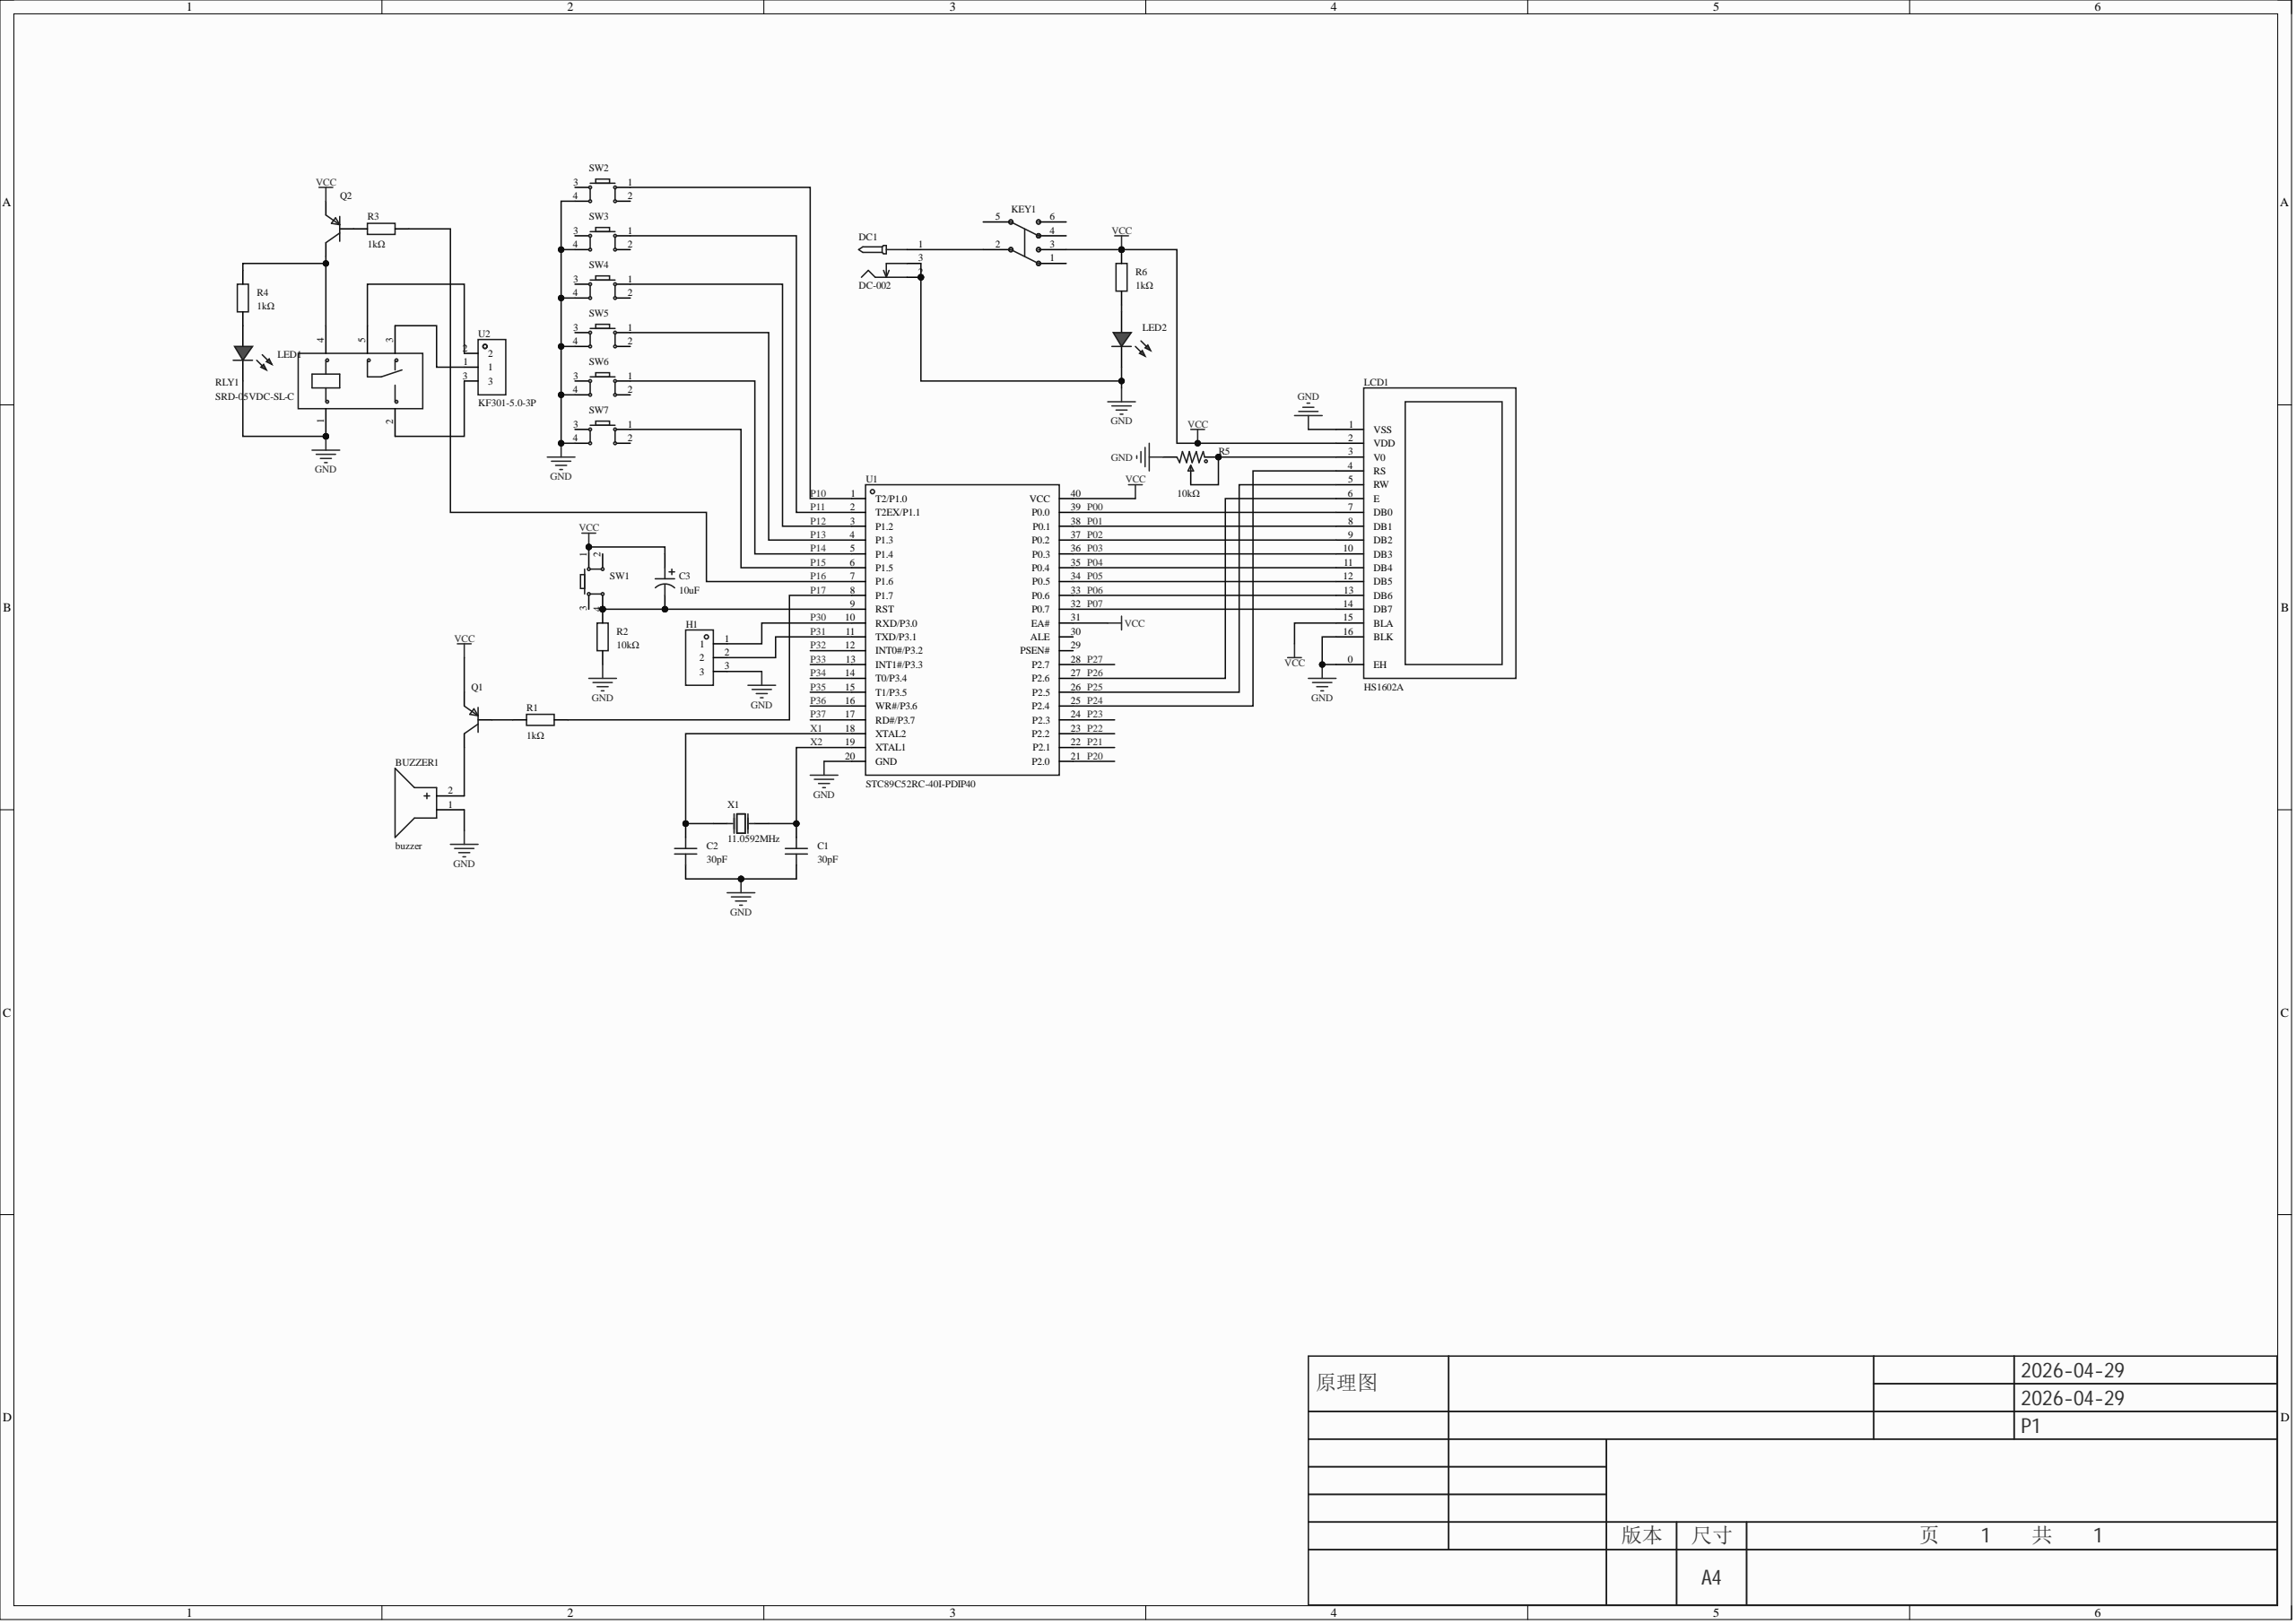Circuit board | Altium Designer | 29 parts | 37 nets
Bill of materials:
Comment,Description,Designator,Footprint,LibRef,Quantity
"buzzer","","BUZZER1","BUZ-TH_BD12.0-P6.00-D0.9-RD","buzzer","1"
"30pF","容值:30pF;精度:±10%;额定电压:25V;温度系数:C0G;","C1, C2","CAP-TH_L3.8-W2.5-P2.54-D0.50","C315C300K3G5TA7301","2"
"10uF","","C3","CAP-TH_BD5.0-P2.00-D0.8-FD-10UF50VC110GL","10UF50VC110GL","1"
"DC-002","","DC1","DC-IN-TH_DC-3510","DC-002","1"
"","","H1","HDR-TH_3P-P2.54-V-M","HDR-M_2.54_1x3P","1"
"无自锁开关 8.5×8.5 无声","6脚，8.5×8.5","KEY1","SW-TH_6P-L8.5-W8.5-P2.54","无自锁开关 8.5×8.5 无声","1"
"HS1602A","主控芯片:SPLC780;尺寸(inch):2;","LCD1","LCD1602","HS1602A","1"
"","","LED1, LED2","LED_TH-3mm","LED_TH-R_3mm","2"
"","","Q1, Q2","S8550P_TO-92","S8550_TO_PNP","2"
"1kΩ","","R1, R3, R4, R6","Res_1/8W","Res_AXIAL-1/8W","4"
"10kΩ","","R2","Res_1/8W","Res_AXIAL-1/8W","1"
"10kΩ","","R5","RES-ADJ-SMD_RM065-V1","RM065-103(10K)","1"
"SRD-05VDC-SL-C","线圈电压:5V;触点形式:一组转换:1C(单刀双掷-转换);触点容量(电阻负载):-;最大切换电压:250V@AC;最大切换电流:15A;","RLY1","RELAY-TH_SRD-XXVDC-XL-C","SRD-05VDC-SL-C","1"
"","","SW1, SW2, SW3, SW4, SW5, SW6, SW7","SW-TH_4P-L6.0-W6.0-P4.50-LS6.5","Key_TH_6x6x6","7"
"STC89C52RC-40I-PDIP40","CPU内核:51家族;CPU最大主频:-;","U1","DIP-40_L52.0-W13.7-P2.54-LS15.2-BL","STC89C52RC-40I-PDIP40","1"
"KF301-5.0-3P","结构:1x3P;间距:5mm;颜色:蓝色;安装方式:直插;排数:1;每排PIN数:3;额定电流:17A;额定电压:250V;线规 - AWG:14~22;线规 - 平方毫米:1.5;工作温度:-30℃~+120℃;","U2","CONN-TH_3P-P5.00_KF301-5.0-3P","KF301-5.0-3P","1"
"11.059MHz","晶振类型:直插晶振;频率:11.059MHz;常温频差:±20ppm;负载电容:30pF;","X1","OSC-TH_L11.1-W4.7-P4.88","9AC11059302060C3","1"
Netlist (Protel format):
[
BUZZER1
BUZ-TH_BD12.0-P6.00-D0.9-RD
buzzer



]
[
C1
CAP-TH_L3.8-W2.5-P2.54-D0.50
30pF



]
[
C2
CAP-TH_L3.8-W2.5-P2.54-D0.50
30pF



]
[
C3
CAP-TH_BD5.0-P2.00-D0.8-FD-10UF50VC110GL
10uF



]
[
DC1
DC-IN-TH_DC-3510
DC-002



]
[
H1
HDR-TH_3P-P2.54-V-M




]
[
KEY1
SW-TH_6P-L8.5-W8.5-P2.54
无自锁开关 8.5×8.5 无声



]
[
LCD1
LCD1602
HS1602A



]
[
LED1
LED_TH-3mm




]
[
LED2
LED_TH-3mm




]
[
Q1
S8550P_TO-92




]
[
Q2
S8550P_TO-92




]
[
R1
Res_1/8W
1kΩ



]
[
R2
Res_1/8W
10kΩ



]
[
R3
Res_1/8W
1kΩ



]
[
R4
Res_1/8W
1kΩ



]
[
R5
RES-ADJ-SMD_RM065-V1
10kΩ



]
[
R6
Res_1/8W
1kΩ



]
[
RLY1
RELAY-TH_SRD-XXVDC-XL-C
SRD-05VDC-SL-C



]
[
SW1
SW-TH_4P-L6.0-W6.0-P4.50-LS6.5




]
[
SW2
SW-TH_4P-L6.0-W6.0-P4.50-LS6.5




]
[
SW3
SW-TH_4P-L6.0-W6.0-P4.50-LS6.5




]
[
SW4
SW-TH_4P-L6.0-W6.0-P4.50-LS6.5




]
[
SW5
SW-TH_4P-L6.0-W6.0-P4.50-LS6.5




]
[
SW6
SW-TH_4P-L6.0-W6.0-P4.50-LS6.5




]
[
SW7
SW-TH_4P-L6.0-W6.0-P4.50-LS6.5




]
[
U1
DIP-40_L52.0-W13.7-P2.54-LS15.2-BL
STC89C52RC-40I-PDIP40



]
[
U2
CONN-TH_3P-P5.00_KF301-5.0-3P
KF301-5.0-3P



]
[
X1
OSC-TH_L11.1-W4.7-P4.88
11.0592MHz



]
(
X2
C1-2
U1-19
X1-2
)
(
X1
C2-2
U1-18
X1-1
)
(
VCC
C3-1
KEY1-3
LCD1-2
LCD1-15
Q1-1
Q2-1
R6-2
SW1-1
U1-31
U1-40
)
(
P31
H1-2
U1-11
)
(
P30
H1-1
U1-10
)
(
P26
LCD1-6
U1-27
)
(
P25
LCD1-5
U1-26
)
(
P24
LCD1-4
U1-25
)
(
P17
R1-2
U1-8
)
(
P16
R3-2
U1-7
)
(
P15
SW7-1
U1-6
)
(
P14
SW6-1
U1-5
)
(
P13
SW5-1
U1-4
)
(
P12
SW4-1
U1-3
)
(
P11
SW3-1
U1-2
)
(
P10
SW2-1
U1-1
)
(
P07
LCD1-14
U1-32
)
(
P06
LCD1-13
U1-33
)
(
P05
LCD1-12
U1-34
)
(
P04
LCD1-11
U1-35
)
(
P03
LCD1-10
U1-36
)
(
P02
LCD1-9
U1-37
)
(
P01
LCD1-8
U1-38
)
(
P00
LCD1-7
U1-39
)
(
NetRLY1_5
RLY1-5
U2-2
)
(
NetRLY1_3
RLY1-3
U2-1
)
(
NetRLY1_2
RLY1-2
U2-3
)
(
NetQ2_3
Q2-3
R4-2
RLY1-4
)
(
NetQ2_2
Q2-2
R3-1
)
(
NetQ1_2
Q1-2
R1-1
)
(
NetLED2_1
LED2-1
R6-1
)
(
NetLED1_1
LED1-1
R4-1
)
(
NetLCD1_3
LCD1-3
R5-1
R5-2
)
(
NetDC1_1
DC1-1
KEY1-2
)
(
NetC3_2
C3-2
R2-2
SW1-4
U1-9
)
(
NetBUZZER1_2
BUZZER1-2
Q1-3
)
(
GND
BUZZER1-1
C1-1
C2-1
DC1-2
DC1-3
H1-3
LCD1-0
LCD1-1
LCD1-16
LED1-2
LED2-2
R2-1
R5-3
RLY1-1
SW2-4
SW3-4
SW4-4
SW5-4
SW6-4
SW7-4
U1-20
)